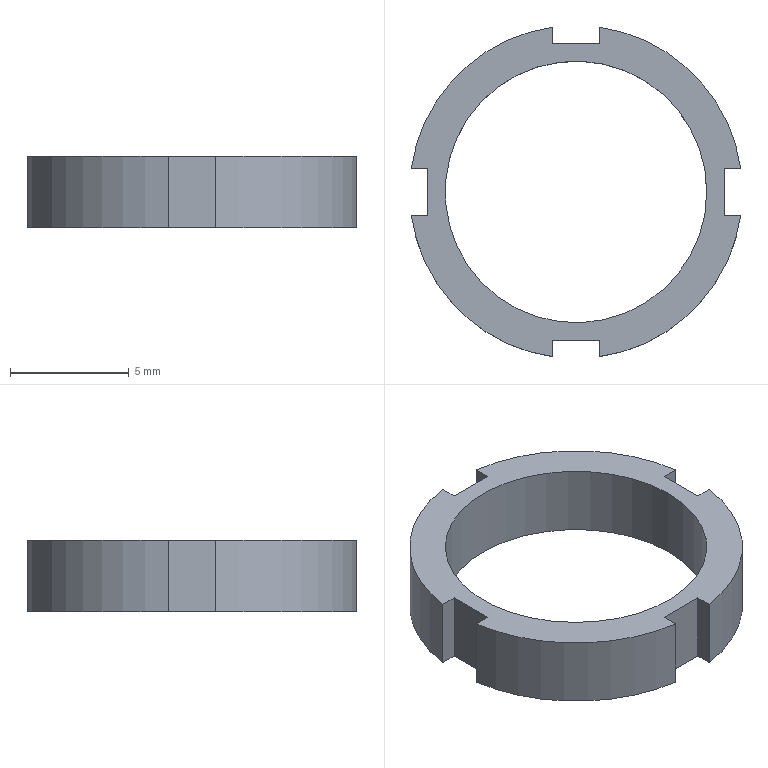Part | NX | features DATUM_CSYS 2, EXTRUDE 1, SKETCH 1 | 1 solid | 19 faces | box 13.856 x 13.856 x 3 mm | volume 159.288 mm3 | plane 14 | cylinder 5 | commonest cylinder face diameters 14 x4 11 x1
STEP:
#1=CARTESIAN_POINT('',(-6.25,-1.,0.));
#2=VERTEX_POINT('',#1);
#3=CARTESIAN_POINT('',(-6.928,-1.,0.));
#4=VERTEX_POINT('',#3);
#5=CARTESIAN_POINT('',(-6.25,-1.,0.));
#6=DIRECTION('',(-1.,0.,0.));
#7=VECTOR('',#6,1000.);
#8=LINE('',#5,#7);
#9=EDGE_CURVE('',#2,#4,#8,.T.);
#10=ORIENTED_EDGE('',*,*,#9,.T.);
#11=CARTESIAN_POINT('',(-6.928,-1.,3.));
#12=VERTEX_POINT('',#11);
#13=CARTESIAN_POINT('',(-6.928,-1.,3.));
#14=DIRECTION('',(0.,0.,-1.));
#15=VECTOR('',#14,1000.);
#16=LINE('',#13,#15);
#17=EDGE_CURVE('',#12,#4,#16,.T.);
#18=ORIENTED_EDGE('',*,*,#17,.F.);
#19=CARTESIAN_POINT('',(-6.25,-1.,3.));
#20=VERTEX_POINT('',#19);
#21=CARTESIAN_POINT('',(-6.25,-1.,3.));
#22=DIRECTION('',(-1.,0.,0.));
#23=VECTOR('',#22,1000.);
#24=LINE('',#21,#23);
#25=EDGE_CURVE('',#20,#12,#24,.T.);
#26=ORIENTED_EDGE('',*,*,#25,.F.);
#27=CARTESIAN_POINT('',(-6.25,-1.,3.));
#28=DIRECTION('',(0.,0.,-1.));
#29=VECTOR('',#28,1000.);
#30=LINE('',#27,#29);
#31=EDGE_CURVE('',#20,#2,#30,.T.);
#32=ORIENTED_EDGE('',*,*,#31,.T.);
#33=EDGE_LOOP('',(#10,#18,#26,#32));
#34=FACE_BOUND('',#33,.T.);
#35=CARTESIAN_POINT('',(-6.25,-1.,3.));
#36=DIRECTION('',(0.,-1.,0.));
#37=DIRECTION('',(1.,0.,0.));
#38=AXIS2_PLACEMENT_3D('',#35,#36,#37);
#39=PLANE('',#38);
#40=ADVANCED_FACE('',(#34),#39,.F.);
#41=CARTESIAN_POINT('',(-1.,-6.928,0.));
#42=VERTEX_POINT('',#41);
#43=CARTESIAN_POINT('',(0.,0.,0.));
#44=DIRECTION('',(0.,0.,1.));
#45=DIRECTION('',(1.,0.,0.));
#46=AXIS2_PLACEMENT_3D('',#43,#44,#45);
#47=CIRCLE('',#46,7.);
#48=EDGE_CURVE('',#4,#42,#47,.T.);
#49=ORIENTED_EDGE('',*,*,#48,.T.);
#50=CARTESIAN_POINT('',(-1.,-6.928,3.));
#51=VERTEX_POINT('',#50);
#52=CARTESIAN_POINT('',(-1.,-6.928,3.));
#53=DIRECTION('',(0.,0.,-1.));
#54=VECTOR('',#53,1000.);
#55=LINE('',#52,#54);
#56=EDGE_CURVE('',#51,#42,#55,.T.);
#57=ORIENTED_EDGE('',*,*,#56,.F.);
#58=CARTESIAN_POINT('',(0.,0.,3.));
#59=DIRECTION('',(0.,0.,1.));
#60=DIRECTION('',(1.,0.,0.));
#61=AXIS2_PLACEMENT_3D('',#58,#59,#60);
#62=CIRCLE('',#61,7.);
#63=EDGE_CURVE('',#12,#51,#62,.T.);
#64=ORIENTED_EDGE('',*,*,#63,.F.);
#65=ORIENTED_EDGE('',*,*,#17,.T.);
#66=EDGE_LOOP('',(#49,#57,#64,#65));
#67=FACE_BOUND('',#66,.T.);
#68=CARTESIAN_POINT('',(0.,0.,3.));
#69=DIRECTION('',(0.,0.,-1.));
#70=DIRECTION('',(-1.,0.,0.));
#71=AXIS2_PLACEMENT_3D('',#68,#69,#70);
#72=CYLINDRICAL_SURFACE('',#71,7.);
#73=ADVANCED_FACE('',(#67),#72,.T.);
#74=CARTESIAN_POINT('',(-1.,-6.25,0.));
#75=VERTEX_POINT('',#74);
#76=CARTESIAN_POINT('',(-1.,-6.928,0.));
#77=DIRECTION('',(0.,1.,0.));
#78=VECTOR('',#77,1000.);
#79=LINE('',#76,#78);
#80=EDGE_CURVE('',#42,#75,#79,.T.);
#81=ORIENTED_EDGE('',*,*,#80,.T.);
#82=CARTESIAN_POINT('',(-1.,-6.25,3.));
#83=VERTEX_POINT('',#82);
#84=CARTESIAN_POINT('',(-1.,-6.25,3.));
#85=DIRECTION('',(0.,0.,-1.));
#86=VECTOR('',#85,1000.);
#87=LINE('',#84,#86);
#88=EDGE_CURVE('',#83,#75,#87,.T.);
#89=ORIENTED_EDGE('',*,*,#88,.F.);
#90=CARTESIAN_POINT('',(-1.,-6.928,3.));
#91=DIRECTION('',(0.,1.,0.));
#92=VECTOR('',#91,1000.);
#93=LINE('',#90,#92);
#94=EDGE_CURVE('',#51,#83,#93,.T.);
#95=ORIENTED_EDGE('',*,*,#94,.F.);
#96=ORIENTED_EDGE('',*,*,#56,.T.);
#97=EDGE_LOOP('',(#81,#89,#95,#96));
#98=FACE_BOUND('',#97,.T.);
#99=CARTESIAN_POINT('',(-1.,-6.928,3.));
#100=DIRECTION('',(-1.,0.,0.));
#101=DIRECTION('',(0.,-1.,0.));
#102=AXIS2_PLACEMENT_3D('',#99,#100,#101);
#103=PLANE('',#102);
#104=ADVANCED_FACE('',(#98),#103,.F.);
#105=CARTESIAN_POINT('',(1.,-6.25,0.));
#106=VERTEX_POINT('',#105);
#107=CARTESIAN_POINT('',(-1.,-6.25,0.));
#108=DIRECTION('',(1.,0.,0.));
#109=VECTOR('',#108,1000.);
#110=LINE('',#107,#109);
#111=EDGE_CURVE('',#75,#106,#110,.T.);
#112=ORIENTED_EDGE('',*,*,#111,.T.);
#113=CARTESIAN_POINT('',(1.,-6.25,3.));
#114=VERTEX_POINT('',#113);
#115=CARTESIAN_POINT('',(1.,-6.25,3.));
#116=DIRECTION('',(0.,0.,-1.));
#117=VECTOR('',#116,1000.);
#118=LINE('',#115,#117);
#119=EDGE_CURVE('',#114,#106,#118,.T.);
#120=ORIENTED_EDGE('',*,*,#119,.F.);
#121=CARTESIAN_POINT('',(-1.,-6.25,3.));
#122=DIRECTION('',(1.,0.,0.));
#123=VECTOR('',#122,1000.);
#124=LINE('',#121,#123);
#125=EDGE_CURVE('',#83,#114,#124,.T.);
#126=ORIENTED_EDGE('',*,*,#125,.F.);
#127=ORIENTED_EDGE('',*,*,#88,.T.);
#128=EDGE_LOOP('',(#112,#120,#126,#127));
#129=FACE_BOUND('',#128,.T.);
#130=CARTESIAN_POINT('',(-1.,-6.25,3.));
#131=DIRECTION('',(0.,1.,0.));
#132=DIRECTION('',(0.,0.,1.));
#133=AXIS2_PLACEMENT_3D('',#130,#131,#132);
#134=PLANE('',#133);
#135=ADVANCED_FACE('',(#129),#134,.F.);
#136=CARTESIAN_POINT('',(1.,-6.928,0.));
#137=VERTEX_POINT('',#136);
#138=CARTESIAN_POINT('',(1.,-6.25,0.));
#139=DIRECTION('',(0.,-1.,0.));
#140=VECTOR('',#139,1000.);
#141=LINE('',#138,#140);
#142=EDGE_CURVE('',#106,#137,#141,.T.);
#143=ORIENTED_EDGE('',*,*,#142,.T.);
#144=CARTESIAN_POINT('',(1.,-6.928,3.));
#145=VERTEX_POINT('',#144);
#146=CARTESIAN_POINT('',(1.,-6.928,3.));
#147=DIRECTION('',(0.,0.,-1.));
#148=VECTOR('',#147,1000.);
#149=LINE('',#146,#148);
#150=EDGE_CURVE('',#145,#137,#149,.T.);
#151=ORIENTED_EDGE('',*,*,#150,.F.);
#152=CARTESIAN_POINT('',(1.,-6.25,3.));
#153=DIRECTION('',(0.,-1.,0.));
#154=VECTOR('',#153,1000.);
#155=LINE('',#152,#154);
#156=EDGE_CURVE('',#114,#145,#155,.T.);
#157=ORIENTED_EDGE('',*,*,#156,.F.);
#158=ORIENTED_EDGE('',*,*,#119,.T.);
#159=EDGE_LOOP('',(#143,#151,#157,#158));
#160=FACE_BOUND('',#159,.T.);
#161=CARTESIAN_POINT('',(1.,-6.25,3.));
#162=DIRECTION('',(1.,0.,0.));
#163=DIRECTION('',(0.,1.,0.));
#164=AXIS2_PLACEMENT_3D('',#161,#162,#163);
#165=PLANE('',#164);
#166=ADVANCED_FACE('',(#160),#165,.F.);
#167=CARTESIAN_POINT('',(6.928,-1.,0.));
#168=VERTEX_POINT('',#167);
#169=CARTESIAN_POINT('',(0.,0.,0.));
#170=DIRECTION('',(0.,0.,1.));
#171=DIRECTION('',(1.,0.,0.));
#172=AXIS2_PLACEMENT_3D('',#169,#170,#171);
#173=CIRCLE('',#172,7.);
#174=EDGE_CURVE('',#137,#168,#173,.T.);
#175=ORIENTED_EDGE('',*,*,#174,.T.);
#176=CARTESIAN_POINT('',(6.928,-1.,3.));
#177=VERTEX_POINT('',#176);
#178=CARTESIAN_POINT('',(6.928,-1.,3.));
#179=DIRECTION('',(0.,0.,-1.));
#180=VECTOR('',#179,1000.);
#181=LINE('',#178,#180);
#182=EDGE_CURVE('',#177,#168,#181,.T.);
#183=ORIENTED_EDGE('',*,*,#182,.F.);
#184=CARTESIAN_POINT('',(0.,0.,3.));
#185=DIRECTION('',(0.,0.,1.));
#186=DIRECTION('',(1.,0.,0.));
#187=AXIS2_PLACEMENT_3D('',#184,#185,#186);
#188=CIRCLE('',#187,7.);
#189=EDGE_CURVE('',#145,#177,#188,.T.);
#190=ORIENTED_EDGE('',*,*,#189,.F.);
#191=ORIENTED_EDGE('',*,*,#150,.T.);
#192=EDGE_LOOP('',(#175,#183,#190,#191));
#193=FACE_BOUND('',#192,.T.);
#194=CARTESIAN_POINT('',(0.,0.,3.));
#195=DIRECTION('',(0.,0.,-1.));
#196=DIRECTION('',(-1.,0.,0.));
#197=AXIS2_PLACEMENT_3D('',#194,#195,#196);
#198=CYLINDRICAL_SURFACE('',#197,7.);
#199=ADVANCED_FACE('',(#193),#198,.T.);
#200=CARTESIAN_POINT('',(6.25,-1.,0.));
#201=VERTEX_POINT('',#200);
#202=CARTESIAN_POINT('',(6.928,-1.,0.));
#203=DIRECTION('',(-1.,0.,0.));
#204=VECTOR('',#203,1000.);
#205=LINE('',#202,#204);
#206=EDGE_CURVE('',#168,#201,#205,.T.);
#207=ORIENTED_EDGE('',*,*,#206,.T.);
#208=CARTESIAN_POINT('',(6.25,-1.,3.));
#209=VERTEX_POINT('',#208);
#210=CARTESIAN_POINT('',(6.25,-1.,3.));
#211=DIRECTION('',(0.,0.,-1.));
#212=VECTOR('',#211,1000.);
#213=LINE('',#210,#212);
#214=EDGE_CURVE('',#209,#201,#213,.T.);
#215=ORIENTED_EDGE('',*,*,#214,.F.);
#216=CARTESIAN_POINT('',(6.928,-1.,3.));
#217=DIRECTION('',(-1.,0.,0.));
#218=VECTOR('',#217,1000.);
#219=LINE('',#216,#218);
#220=EDGE_CURVE('',#177,#209,#219,.T.);
#221=ORIENTED_EDGE('',*,*,#220,.F.);
#222=ORIENTED_EDGE('',*,*,#182,.T.);
#223=EDGE_LOOP('',(#207,#215,#221,#222));
#224=FACE_BOUND('',#223,.T.);
#225=CARTESIAN_POINT('',(6.928,-1.,3.));
#226=DIRECTION('',(0.,-1.,0.));
#227=DIRECTION('',(1.,0.,0.));
#228=AXIS2_PLACEMENT_3D('',#225,#226,#227);
#229=PLANE('',#228);
#230=ADVANCED_FACE('',(#224),#229,.F.);
#231=CARTESIAN_POINT('',(6.25,1.,0.));
#232=VERTEX_POINT('',#231);
#233=CARTESIAN_POINT('',(6.25,-1.,0.));
#234=DIRECTION('',(0.,1.,0.));
#235=VECTOR('',#234,1000.);
#236=LINE('',#233,#235);
#237=EDGE_CURVE('',#201,#232,#236,.T.);
#238=ORIENTED_EDGE('',*,*,#237,.T.);
#239=CARTESIAN_POINT('',(6.25,1.,3.));
#240=VERTEX_POINT('',#239);
#241=CARTESIAN_POINT('',(6.25,1.,3.));
#242=DIRECTION('',(0.,0.,-1.));
#243=VECTOR('',#242,1000.);
#244=LINE('',#241,#243);
#245=EDGE_CURVE('',#240,#232,#244,.T.);
#246=ORIENTED_EDGE('',*,*,#245,.F.);
#247=CARTESIAN_POINT('',(6.25,-1.,3.));
#248=DIRECTION('',(0.,1.,0.));
#249=VECTOR('',#248,1000.);
#250=LINE('',#247,#249);
#251=EDGE_CURVE('',#209,#240,#250,.T.);
#252=ORIENTED_EDGE('',*,*,#251,.F.);
#253=ORIENTED_EDGE('',*,*,#214,.T.);
#254=EDGE_LOOP('',(#238,#246,#252,#253));
#255=FACE_BOUND('',#254,.T.);
#256=CARTESIAN_POINT('',(6.25,-1.,3.));
#257=DIRECTION('',(-1.,0.,0.));
#258=DIRECTION('',(0.,0.,1.));
#259=AXIS2_PLACEMENT_3D('',#256,#257,#258);
#260=PLANE('',#259);
#261=ADVANCED_FACE('',(#255),#260,.F.);
#262=CARTESIAN_POINT('',(6.928,1.,0.));
#263=VERTEX_POINT('',#262);
#264=CARTESIAN_POINT('',(6.25,1.,0.));
#265=DIRECTION('',(1.,0.,0.));
#266=VECTOR('',#265,1000.);
#267=LINE('',#264,#266);
#268=EDGE_CURVE('',#232,#263,#267,.T.);
#269=ORIENTED_EDGE('',*,*,#268,.T.);
#270=CARTESIAN_POINT('',(6.928,1.,3.));
#271=VERTEX_POINT('',#270);
#272=CARTESIAN_POINT('',(6.928,1.,3.));
#273=DIRECTION('',(0.,0.,-1.));
#274=VECTOR('',#273,1000.);
#275=LINE('',#272,#274);
#276=EDGE_CURVE('',#271,#263,#275,.T.);
#277=ORIENTED_EDGE('',*,*,#276,.F.);
#278=CARTESIAN_POINT('',(6.25,1.,3.));
#279=DIRECTION('',(1.,0.,0.));
#280=VECTOR('',#279,1000.);
#281=LINE('',#278,#280);
#282=EDGE_CURVE('',#240,#271,#281,.T.);
#283=ORIENTED_EDGE('',*,*,#282,.F.);
#284=ORIENTED_EDGE('',*,*,#245,.T.);
#285=EDGE_LOOP('',(#269,#277,#283,#284));
#286=FACE_BOUND('',#285,.T.);
#287=CARTESIAN_POINT('',(6.25,1.,3.));
#288=DIRECTION('',(0.,1.,0.));
#289=DIRECTION('',(-1.,0.,0.));
#290=AXIS2_PLACEMENT_3D('',#287,#288,#289);
#291=PLANE('',#290);
#292=ADVANCED_FACE('',(#286),#291,.F.);
#293=CARTESIAN_POINT('',(1.,6.928,0.));
#294=VERTEX_POINT('',#293);
#295=CARTESIAN_POINT('',(0.,0.,0.));
#296=DIRECTION('',(0.,0.,1.));
#297=DIRECTION('',(1.,0.,0.));
#298=AXIS2_PLACEMENT_3D('',#295,#296,#297);
#299=CIRCLE('',#298,7.);
#300=EDGE_CURVE('',#263,#294,#299,.T.);
#301=ORIENTED_EDGE('',*,*,#300,.T.);
#302=CARTESIAN_POINT('',(1.,6.928,3.));
#303=VERTEX_POINT('',#302);
#304=CARTESIAN_POINT('',(1.,6.928,3.));
#305=DIRECTION('',(0.,0.,-1.));
#306=VECTOR('',#305,1000.);
#307=LINE('',#304,#306);
#308=EDGE_CURVE('',#303,#294,#307,.T.);
#309=ORIENTED_EDGE('',*,*,#308,.F.);
#310=CARTESIAN_POINT('',(0.,0.,3.));
#311=DIRECTION('',(0.,0.,1.));
#312=DIRECTION('',(1.,0.,0.));
#313=AXIS2_PLACEMENT_3D('',#310,#311,#312);
#314=CIRCLE('',#313,7.);
#315=EDGE_CURVE('',#271,#303,#314,.T.);
#316=ORIENTED_EDGE('',*,*,#315,.F.);
#317=ORIENTED_EDGE('',*,*,#276,.T.);
#318=EDGE_LOOP('',(#301,#309,#316,#317));
#319=FACE_BOUND('',#318,.T.);
#320=CARTESIAN_POINT('',(0.,0.,3.));
#321=DIRECTION('',(0.,0.,-1.));
#322=DIRECTION('',(-1.,0.,0.));
#323=AXIS2_PLACEMENT_3D('',#320,#321,#322);
#324=CYLINDRICAL_SURFACE('',#323,7.);
#325=ADVANCED_FACE('',(#319),#324,.T.);
#326=CARTESIAN_POINT('',(1.,6.25,0.));
#327=VERTEX_POINT('',#326);
#328=CARTESIAN_POINT('',(1.,6.928,0.));
#329=DIRECTION('',(0.,-1.,0.));
#330=VECTOR('',#329,1000.);
#331=LINE('',#328,#330);
#332=EDGE_CURVE('',#294,#327,#331,.T.);
#333=ORIENTED_EDGE('',*,*,#332,.T.);
#334=CARTESIAN_POINT('',(1.,6.25,3.));
#335=VERTEX_POINT('',#334);
#336=CARTESIAN_POINT('',(1.,6.25,3.));
#337=DIRECTION('',(0.,0.,-1.));
#338=VECTOR('',#337,1000.);
#339=LINE('',#336,#338);
#340=EDGE_CURVE('',#335,#327,#339,.T.);
#341=ORIENTED_EDGE('',*,*,#340,.F.);
#342=CARTESIAN_POINT('',(1.,6.928,3.));
#343=DIRECTION('',(0.,-1.,0.));
#344=VECTOR('',#343,1000.);
#345=LINE('',#342,#344);
#346=EDGE_CURVE('',#303,#335,#345,.T.);
#347=ORIENTED_EDGE('',*,*,#346,.F.);
#348=ORIENTED_EDGE('',*,*,#308,.T.);
#349=EDGE_LOOP('',(#333,#341,#347,#348));
#350=FACE_BOUND('',#349,.T.);
#351=CARTESIAN_POINT('',(1.,6.928,3.));
#352=DIRECTION('',(1.,0.,0.));
#353=DIRECTION('',(0.,1.,0.));
#354=AXIS2_PLACEMENT_3D('',#351,#352,#353);
#355=PLANE('',#354);
#356=ADVANCED_FACE('',(#350),#355,.F.);
#357=CARTESIAN_POINT('',(-1.,6.25,0.));
#358=VERTEX_POINT('',#357);
#359=CARTESIAN_POINT('',(1.,6.25,0.));
#360=DIRECTION('',(-1.,0.,0.));
#361=VECTOR('',#360,1000.);
#362=LINE('',#359,#361);
#363=EDGE_CURVE('',#327,#358,#362,.T.);
#364=ORIENTED_EDGE('',*,*,#363,.T.);
#365=CARTESIAN_POINT('',(-1.,6.25,3.));
#366=VERTEX_POINT('',#365);
#367=CARTESIAN_POINT('',(-1.,6.25,3.));
#368=DIRECTION('',(0.,0.,-1.));
#369=VECTOR('',#368,1000.);
#370=LINE('',#367,#369);
#371=EDGE_CURVE('',#366,#358,#370,.T.);
#372=ORIENTED_EDGE('',*,*,#371,.F.);
#373=CARTESIAN_POINT('',(1.,6.25,3.));
#374=DIRECTION('',(-1.,0.,0.));
#375=VECTOR('',#374,1000.);
#376=LINE('',#373,#375);
#377=EDGE_CURVE('',#335,#366,#376,.T.);
#378=ORIENTED_EDGE('',*,*,#377,.F.);
#379=ORIENTED_EDGE('',*,*,#340,.T.);
#380=EDGE_LOOP('',(#364,#372,#378,#379));
#381=FACE_BOUND('',#380,.T.);
#382=CARTESIAN_POINT('',(1.,6.25,3.));
#383=DIRECTION('',(0.,-1.,0.));
#384=DIRECTION('',(0.,0.,-1.));
#385=AXIS2_PLACEMENT_3D('',#382,#383,#384);
#386=PLANE('',#385);
#387=ADVANCED_FACE('',(#381),#386,.F.);
#388=CARTESIAN_POINT('',(-1.,6.928,0.));
#389=VERTEX_POINT('',#388);
#390=CARTESIAN_POINT('',(-1.,6.25,0.));
#391=DIRECTION('',(0.,1.,0.));
#392=VECTOR('',#391,1000.);
#393=LINE('',#390,#392);
#394=EDGE_CURVE('',#358,#389,#393,.T.);
#395=ORIENTED_EDGE('',*,*,#394,.T.);
#396=CARTESIAN_POINT('',(-1.,6.928,3.));
#397=VERTEX_POINT('',#396);
#398=CARTESIAN_POINT('',(-1.,6.928,3.));
#399=DIRECTION('',(0.,0.,-1.));
#400=VECTOR('',#399,1000.);
#401=LINE('',#398,#400);
#402=EDGE_CURVE('',#397,#389,#401,.T.);
#403=ORIENTED_EDGE('',*,*,#402,.F.);
#404=CARTESIAN_POINT('',(-1.,6.25,3.));
#405=DIRECTION('',(0.,1.,0.));
#406=VECTOR('',#405,1000.);
#407=LINE('',#404,#406);
#408=EDGE_CURVE('',#366,#397,#407,.T.);
#409=ORIENTED_EDGE('',*,*,#408,.F.);
#410=ORIENTED_EDGE('',*,*,#371,.T.);
#411=EDGE_LOOP('',(#395,#403,#409,#410));
#412=FACE_BOUND('',#411,.T.);
#413=CARTESIAN_POINT('',(-1.,6.25,3.));
#414=DIRECTION('',(-1.,0.,0.));
#415=DIRECTION('',(0.,-1.,0.));
#416=AXIS2_PLACEMENT_3D('',#413,#414,#415);
#417=PLANE('',#416);
#418=ADVANCED_FACE('',(#412),#417,.F.);
#419=CARTESIAN_POINT('',(-6.928,1.,0.));
#420=VERTEX_POINT('',#419);
#421=CARTESIAN_POINT('',(0.,0.,0.));
#422=DIRECTION('',(0.,0.,1.));
#423=DIRECTION('',(1.,0.,0.));
#424=AXIS2_PLACEMENT_3D('',#421,#422,#423);
#425=CIRCLE('',#424,7.);
#426=EDGE_CURVE('',#389,#420,#425,.T.);
#427=ORIENTED_EDGE('',*,*,#426,.T.);
#428=CARTESIAN_POINT('',(-6.928,1.,3.));
#429=VERTEX_POINT('',#428);
#430=CARTESIAN_POINT('',(-6.928,1.,3.));
#431=DIRECTION('',(0.,0.,-1.));
#432=VECTOR('',#431,1000.);
#433=LINE('',#430,#432);
#434=EDGE_CURVE('',#429,#420,#433,.T.);
#435=ORIENTED_EDGE('',*,*,#434,.F.);
#436=CARTESIAN_POINT('',(0.,0.,3.));
#437=DIRECTION('',(0.,0.,1.));
#438=DIRECTION('',(1.,0.,0.));
#439=AXIS2_PLACEMENT_3D('',#436,#437,#438);
#440=CIRCLE('',#439,7.);
#441=EDGE_CURVE('',#397,#429,#440,.T.);
#442=ORIENTED_EDGE('',*,*,#441,.F.);
#443=ORIENTED_EDGE('',*,*,#402,.T.);
#444=EDGE_LOOP('',(#427,#435,#442,#443));
#445=FACE_BOUND('',#444,.T.);
#446=CARTESIAN_POINT('',(0.,0.,3.));
#447=DIRECTION('',(0.,0.,-1.));
#448=DIRECTION('',(-1.,0.,0.));
#449=AXIS2_PLACEMENT_3D('',#446,#447,#448);
#450=CYLINDRICAL_SURFACE('',#449,7.);
#451=ADVANCED_FACE('',(#445),#450,.T.);
#452=CARTESIAN_POINT('',(-6.25,1.,0.));
#453=VERTEX_POINT('',#452);
#454=CARTESIAN_POINT('',(-6.928,1.,0.));
#455=DIRECTION('',(1.,0.,0.));
#456=VECTOR('',#455,1000.);
#457=LINE('',#454,#456);
#458=EDGE_CURVE('',#420,#453,#457,.T.);
#459=ORIENTED_EDGE('',*,*,#458,.T.);
#460=CARTESIAN_POINT('',(-6.25,1.,3.));
#461=VERTEX_POINT('',#460);
#462=CARTESIAN_POINT('',(-6.25,1.,3.));
#463=DIRECTION('',(0.,0.,-1.));
#464=VECTOR('',#463,1000.);
#465=LINE('',#462,#464);
#466=EDGE_CURVE('',#461,#453,#465,.T.);
#467=ORIENTED_EDGE('',*,*,#466,.F.);
#468=CARTESIAN_POINT('',(-6.928,1.,3.));
#469=DIRECTION('',(1.,0.,0.));
#470=VECTOR('',#469,1000.);
#471=LINE('',#468,#470);
#472=EDGE_CURVE('',#429,#461,#471,.T.);
#473=ORIENTED_EDGE('',*,*,#472,.F.);
#474=ORIENTED_EDGE('',*,*,#434,.T.);
#475=EDGE_LOOP('',(#459,#467,#473,#474));
#476=FACE_BOUND('',#475,.T.);
#477=CARTESIAN_POINT('',(-6.928,1.,3.));
#478=DIRECTION('',(0.,1.,0.));
#479=DIRECTION('',(-1.,0.,0.));
#480=AXIS2_PLACEMENT_3D('',#477,#478,#479);
#481=PLANE('',#480);
#482=ADVANCED_FACE('',(#476),#481,.F.);
#483=CARTESIAN_POINT('',(-6.25,1.,0.));
#484=DIRECTION('',(0.,-1.,0.));
#485=VECTOR('',#484,1000.);
#486=LINE('',#483,#485);
#487=EDGE_CURVE('',#453,#2,#486,.T.);
#488=ORIENTED_EDGE('',*,*,#487,.T.);
#489=ORIENTED_EDGE('',*,*,#31,.F.);
#490=CARTESIAN_POINT('',(-6.25,1.,3.));
#491=DIRECTION('',(0.,-1.,0.));
#492=VECTOR('',#491,1000.);
#493=LINE('',#490,#492);
#494=EDGE_CURVE('',#461,#20,#493,.T.);
#495=ORIENTED_EDGE('',*,*,#494,.F.);
#496=ORIENTED_EDGE('',*,*,#466,.T.);
#497=EDGE_LOOP('',(#488,#489,#495,#496));
#498=FACE_BOUND('',#497,.T.);
#499=CARTESIAN_POINT('',(-6.25,1.,3.));
#500=DIRECTION('',(1.,0.,0.));
#501=DIRECTION('',(0.,0.,-1.));
#502=AXIS2_PLACEMENT_3D('',#499,#500,#501);
#503=PLANE('',#502);
#504=ADVANCED_FACE('',(#498),#503,.F.);
#505=CARTESIAN_POINT('',(5.5,0.,3.));
#506=VERTEX_POINT('',#505);
#507=CARTESIAN_POINT('',(0.,0.,3.));
#508=DIRECTION('',(0.,0.,1.));
#509=DIRECTION('',(1.,0.,0.));
#510=AXIS2_PLACEMENT_3D('',#507,#508,#509);
#511=CIRCLE('',#510,5.5);
#512=EDGE_CURVE('',#506,#506,#511,.T.);
#513=ORIENTED_EDGE('',*,*,#512,.T.);
#514=EDGE_LOOP('',(#513));
#515=FACE_BOUND('',#514,.T.);
#516=CARTESIAN_POINT('',(5.5,0.,0.));
#517=VERTEX_POINT('',#516);
#518=CARTESIAN_POINT('',(0.,0.,0.));
#519=DIRECTION('',(0.,0.,1.));
#520=DIRECTION('',(1.,0.,0.));
#521=AXIS2_PLACEMENT_3D('',#518,#519,#520);
#522=CIRCLE('',#521,5.5);
#523=EDGE_CURVE('',#517,#517,#522,.T.);
#524=ORIENTED_EDGE('',*,*,#523,.F.);
#525=EDGE_LOOP('',(#524));
#526=FACE_BOUND('',#525,.T.);
#527=CARTESIAN_POINT('',(0.,0.,3.));
#528=DIRECTION('',(0.,0.,-1.));
#529=DIRECTION('',(-1.,0.,0.));
#530=AXIS2_PLACEMENT_3D('',#527,#528,#529);
#531=CYLINDRICAL_SURFACE('',#530,5.5);
#532=ADVANCED_FACE('',(#515,#526),#531,.F.);
#533=ORIENTED_EDGE('',*,*,#25,.T.);
#534=ORIENTED_EDGE('',*,*,#63,.T.);
#535=ORIENTED_EDGE('',*,*,#94,.T.);
#536=ORIENTED_EDGE('',*,*,#125,.T.);
#537=ORIENTED_EDGE('',*,*,#156,.T.);
#538=ORIENTED_EDGE('',*,*,#189,.T.);
#539=ORIENTED_EDGE('',*,*,#220,.T.);
#540=ORIENTED_EDGE('',*,*,#251,.T.);
#541=ORIENTED_EDGE('',*,*,#282,.T.);
#542=ORIENTED_EDGE('',*,*,#315,.T.);
#543=ORIENTED_EDGE('',*,*,#346,.T.);
#544=ORIENTED_EDGE('',*,*,#377,.T.);
#545=ORIENTED_EDGE('',*,*,#408,.T.);
#546=ORIENTED_EDGE('',*,*,#441,.T.);
#547=ORIENTED_EDGE('',*,*,#472,.T.);
#548=ORIENTED_EDGE('',*,*,#494,.T.);
#549=EDGE_LOOP('',(#533,#534,#535,#536,#537,#538,#539,#540,#541,#542,#543,#544,#545,#546,#547,#548));
#550=FACE_BOUND('',#549,.T.);
#551=ORIENTED_EDGE('',*,*,#512,.F.);
#552=EDGE_LOOP('',(#551));
#553=FACE_BOUND('',#552,.T.);
#554=CARTESIAN_POINT('',(0.,0.,3.));
#555=DIRECTION('',(0.,0.,1.));
#556=DIRECTION('',(1.,0.,0.));
#557=AXIS2_PLACEMENT_3D('',#554,#555,#556);
#558=PLANE('',#557);
#559=ADVANCED_FACE('',(#550,#553),#558,.T.);
#560=ORIENTED_EDGE('',*,*,#9,.F.);
#561=ORIENTED_EDGE('',*,*,#487,.F.);
#562=ORIENTED_EDGE('',*,*,#458,.F.);
#563=ORIENTED_EDGE('',*,*,#426,.F.);
#564=ORIENTED_EDGE('',*,*,#394,.F.);
#565=ORIENTED_EDGE('',*,*,#363,.F.);
#566=ORIENTED_EDGE('',*,*,#332,.F.);
#567=ORIENTED_EDGE('',*,*,#300,.F.);
#568=ORIENTED_EDGE('',*,*,#268,.F.);
#569=ORIENTED_EDGE('',*,*,#237,.F.);
#570=ORIENTED_EDGE('',*,*,#206,.F.);
#571=ORIENTED_EDGE('',*,*,#174,.F.);
#572=ORIENTED_EDGE('',*,*,#142,.F.);
#573=ORIENTED_EDGE('',*,*,#111,.F.);
#574=ORIENTED_EDGE('',*,*,#80,.F.);
#575=ORIENTED_EDGE('',*,*,#48,.F.);
#576=EDGE_LOOP('',(#560,#561,#562,#563,#564,#565,#566,#567,#568,#569,#570,#571,#572,#573,#574,#575));
#577=FACE_BOUND('',#576,.T.);
#578=ORIENTED_EDGE('',*,*,#523,.T.);
#579=EDGE_LOOP('',(#578));
#580=FACE_BOUND('',#579,.T.);
#581=CARTESIAN_POINT('',(0.,0.,0.));
#582=DIRECTION('',(0.,0.,1.));
#583=DIRECTION('',(1.,0.,0.));
#584=AXIS2_PLACEMENT_3D('',#581,#582,#583);
#585=PLANE('',#584);
#586=ADVANCED_FACE('',(#577,#580),#585,.F.);
#587=CLOSED_SHELL('',(#40,#73,#104,#135,#166,#199,#230,#261,#292,#325,#356,#387,#418,#451,#482,#504,#532,#559,#586));
#588=MANIFOLD_SOLID_BREP('',#587);
#589=(LENGTH_UNIT()NAMED_UNIT(*)SI_UNIT(.MILLI.,.METRE.));
#590=UNCERTAINTY_MEASURE_WITH_UNIT(LENGTH_MEASURE(0.00001),#589,'','');
#591=(NAMED_UNIT(*)PLANE_ANGLE_UNIT()SI_UNIT($,.RADIAN.));
#592=(NAMED_UNIT(*)SI_UNIT($,.STERADIAN.)SOLID_ANGLE_UNIT());
#593=(GEOMETRIC_REPRESENTATION_CONTEXT(3)GLOBAL_UNCERTAINTY_ASSIGNED_CONTEXT((#590))GLOBAL_UNIT_ASSIGNED_CONTEXT((#589,#591,#592))REPRESENTATION_CONTEXT('',''));
#594=ADVANCED_BREP_SHAPE_REPRESENTATION('',(#588),#593);